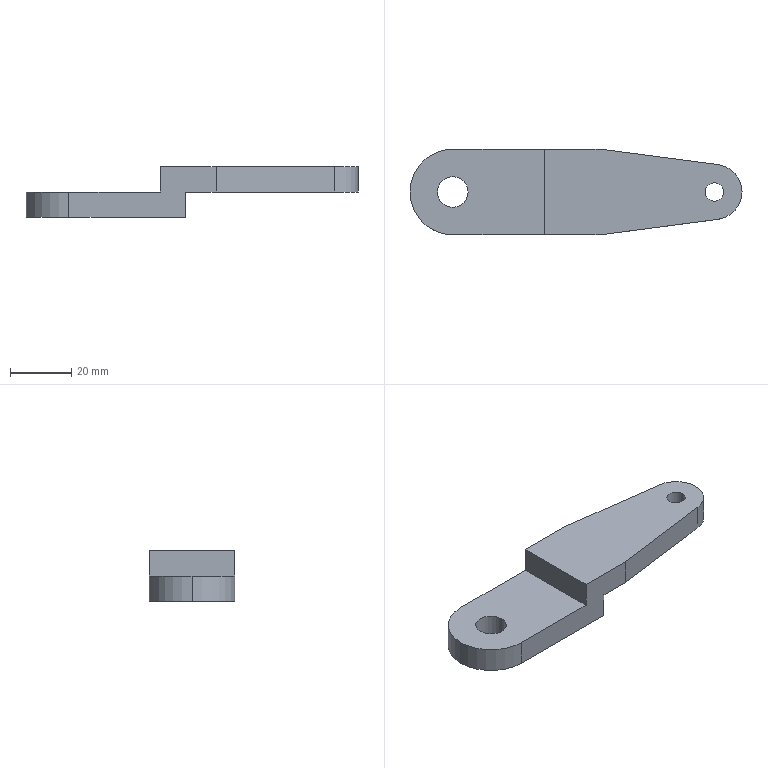Part | SolidWorks | features Extrusion 1, ICE 1 | 1 solid | 17 faces | box 108.5 x 28 x 16.6 mm | volume 22997 mm3 | plane 10 | cylinder 7 | commonest cylinder face diameters 6 x2 10 x2 28 x2 18 x1
STEP:
#1=CARTESIAN_POINT('',(52.6,0.,16.6));
#2=VERTEX_POINT('',#1);
#3=CARTESIAN_POINT('',(58.6,0.,16.6));
#4=VERTEX_POINT('',#3);
#5=CARTESIAN_POINT('',(55.6,0.,16.6));
#6=DIRECTION('',(0.,0.,1.));
#7=DIRECTION('',(1.,0.,0.));
#8=AXIS2_PLACEMENT_3D('',#5,#6,#7);
#9=CIRCLE('',#8,3.);
#10=EDGE_CURVE('',#2,#4,#9,.T.);
#11=ORIENTED_EDGE('',*,*,#10,.T.);
#12=CARTESIAN_POINT('',(58.6,0.,8.3));
#13=VERTEX_POINT('',#12);
#14=CARTESIAN_POINT('',(58.6,0.,16.6));
#15=DIRECTION('',(0.,0.,-1.));
#16=VECTOR('',#15,1000.);
#17=LINE('',#14,#16);
#18=EDGE_CURVE('',#4,#13,#17,.T.);
#19=ORIENTED_EDGE('',*,*,#18,.T.);
#20=CARTESIAN_POINT('',(52.6,0.,8.3));
#21=VERTEX_POINT('',#20);
#22=CARTESIAN_POINT('',(55.6,0.,8.3));
#23=DIRECTION('',(0.,0.,1.));
#24=DIRECTION('',(1.,0.,0.));
#25=AXIS2_PLACEMENT_3D('',#22,#23,#24);
#26=CIRCLE('',#25,3.);
#27=EDGE_CURVE('',#21,#13,#26,.T.);
#28=ORIENTED_EDGE('',*,*,#27,.F.);
#29=CARTESIAN_POINT('',(52.6,0.,16.6));
#30=DIRECTION('',(0.,0.,-1.));
#31=VECTOR('',#30,1000.);
#32=LINE('',#29,#31);
#33=EDGE_CURVE('',#2,#21,#32,.T.);
#34=ORIENTED_EDGE('',*,*,#33,.F.);
#35=EDGE_LOOP('',(#11,#19,#28,#34));
#36=FACE_OUTER_BOUND('',#35,.T.);
#37=CARTESIAN_POINT('',(55.6,0.,16.6));
#38=DIRECTION('',(0.,0.,-1.));
#39=DIRECTION('',(-1.,0.,0.));
#40=AXIS2_PLACEMENT_3D('',#37,#38,#39);
#41=CYLINDRICAL_SURFACE('',#40,3.);
#42=ADVANCED_FACE('',(#36),#41,.F.);
#43=CARTESIAN_POINT('',(-34.9,0.,8.3));
#44=VERTEX_POINT('',#43);
#45=CARTESIAN_POINT('',(-24.9,0.,8.3));
#46=VERTEX_POINT('',#45);
#47=CARTESIAN_POINT('',(-29.9,0.,8.3));
#48=DIRECTION('',(0.,0.,1.));
#49=DIRECTION('',(1.,0.,0.));
#50=AXIS2_PLACEMENT_3D('',#47,#48,#49);
#51=CIRCLE('',#50,5.);
#52=EDGE_CURVE('',#44,#46,#51,.T.);
#53=ORIENTED_EDGE('',*,*,#52,.T.);
#54=CARTESIAN_POINT('',(-24.9,0.,0.));
#55=VERTEX_POINT('',#54);
#56=CARTESIAN_POINT('',(-24.9,0.,8.3));
#57=DIRECTION('',(0.,0.,-1.));
#58=VECTOR('',#57,1000.);
#59=LINE('',#56,#58);
#60=EDGE_CURVE('',#46,#55,#59,.T.);
#61=ORIENTED_EDGE('',*,*,#60,.T.);
#62=CARTESIAN_POINT('',(-34.9,0.,0.));
#63=VERTEX_POINT('',#62);
#64=CARTESIAN_POINT('',(-29.9,0.,0.));
#65=DIRECTION('',(0.,0.,1.));
#66=DIRECTION('',(1.,0.,0.));
#67=AXIS2_PLACEMENT_3D('',#64,#65,#66);
#68=CIRCLE('',#67,5.);
#69=EDGE_CURVE('',#63,#55,#68,.T.);
#70=ORIENTED_EDGE('',*,*,#69,.F.);
#71=CARTESIAN_POINT('',(-34.9,0.,8.3));
#72=DIRECTION('',(0.,0.,-1.));
#73=VECTOR('',#72,1000.);
#74=LINE('',#71,#73);
#75=EDGE_CURVE('',#44,#63,#74,.T.);
#76=ORIENTED_EDGE('',*,*,#75,.F.);
#77=EDGE_LOOP('',(#53,#61,#70,#76));
#78=FACE_OUTER_BOUND('',#77,.T.);
#79=CARTESIAN_POINT('',(-29.9,0.,8.3));
#80=DIRECTION('',(0.,0.,-1.));
#81=DIRECTION('',(-1.,0.,0.));
#82=AXIS2_PLACEMENT_3D('',#79,#80,#81);
#83=CYLINDRICAL_SURFACE('',#82,5.);
#84=ADVANCED_FACE('',(#78),#83,.F.);
#85=CARTESIAN_POINT('',(-43.9,0.,8.3));
#86=VERTEX_POINT('',#85);
#87=CARTESIAN_POINT('',(-29.9,-14.,8.3));
#88=VERTEX_POINT('',#87);
#89=CARTESIAN_POINT('',(-29.9,0.,8.3));
#90=DIRECTION('',(0.,0.,1.));
#91=DIRECTION('',(1.,0.,0.));
#92=AXIS2_PLACEMENT_3D('',#89,#90,#91);
#93=CIRCLE('',#92,14.);
#94=EDGE_CURVE('',#86,#88,#93,.T.);
#95=ORIENTED_EDGE('',*,*,#94,.F.);
#96=CARTESIAN_POINT('',(-43.9,0.,0.));
#97=VERTEX_POINT('',#96);
#98=CARTESIAN_POINT('',(-43.9,0.,8.3));
#99=DIRECTION('',(0.,0.,-1.));
#100=VECTOR('',#99,1000.);
#101=LINE('',#98,#100);
#102=EDGE_CURVE('',#86,#97,#101,.T.);
#103=ORIENTED_EDGE('',*,*,#102,.T.);
#104=CARTESIAN_POINT('',(-29.9,-14.,0.));
#105=VERTEX_POINT('',#104);
#106=CARTESIAN_POINT('',(-29.9,0.,0.));
#107=DIRECTION('',(0.,0.,1.));
#108=DIRECTION('',(1.,0.,0.));
#109=AXIS2_PLACEMENT_3D('',#106,#107,#108);
#110=CIRCLE('',#109,14.);
#111=EDGE_CURVE('',#97,#105,#110,.T.);
#112=ORIENTED_EDGE('',*,*,#111,.T.);
#113=CARTESIAN_POINT('',(-29.9,-14.,8.3));
#114=DIRECTION('',(0.,0.,-1.));
#115=VECTOR('',#114,1000.);
#116=LINE('',#113,#115);
#117=EDGE_CURVE('',#88,#105,#116,.T.);
#118=ORIENTED_EDGE('',*,*,#117,.F.);
#119=EDGE_LOOP('',(#95,#103,#112,#118));
#120=FACE_OUTER_BOUND('',#119,.T.);
#121=CARTESIAN_POINT('',(-29.9,0.,8.3));
#122=DIRECTION('',(0.,0.,-1.));
#123=DIRECTION('',(-1.,0.,0.));
#124=AXIS2_PLACEMENT_3D('',#121,#122,#123);
#125=CYLINDRICAL_SURFACE('',#124,14.);
#126=ADVANCED_FACE('',(#120),#125,.T.);
#127=CARTESIAN_POINT('',(-29.9,14.,0.));
#128=VERTEX_POINT('',#127);
#129=CARTESIAN_POINT('',(8.3,14.,0.));
#130=VERTEX_POINT('',#129);
#131=CARTESIAN_POINT('',(0.,14.,0.));
#132=DIRECTION('',(1.,0.,0.));
#133=VECTOR('',#132,1000.);
#134=LINE('',#131,#133);
#135=EDGE_CURVE('',#128,#130,#134,.T.);
#136=ORIENTED_EDGE('',*,*,#135,.F.);
#137=CARTESIAN_POINT('',(-29.9,14.,8.3));
#138=VERTEX_POINT('',#137);
#139=CARTESIAN_POINT('',(-29.9,14.,8.3));
#140=DIRECTION('',(0.,0.,-1.));
#141=VECTOR('',#140,1000.);
#142=LINE('',#139,#141);
#143=EDGE_CURVE('',#138,#128,#142,.T.);
#144=ORIENTED_EDGE('',*,*,#143,.F.);
#145=CARTESIAN_POINT('',(0.,14.,8.3));
#146=VERTEX_POINT('',#145);
#147=CARTESIAN_POINT('',(0.,14.,8.3));
#148=DIRECTION('',(1.,0.,0.));
#149=VECTOR('',#148,1000.);
#150=LINE('',#147,#149);
#151=EDGE_CURVE('',#138,#146,#150,.T.);
#152=ORIENTED_EDGE('',*,*,#151,.T.);
#153=CARTESIAN_POINT('',(0.,14.,16.6));
#154=VERTEX_POINT('',#153);
#155=CARTESIAN_POINT('',(0.,14.,16.6));
#156=DIRECTION('',(0.,0.,-1.));
#157=VECTOR('',#156,1000.);
#158=LINE('',#155,#157);
#159=EDGE_CURVE('',#154,#146,#158,.T.);
#160=ORIENTED_EDGE('',*,*,#159,.F.);
#161=CARTESIAN_POINT('',(18.211,14.,16.6));
#162=VERTEX_POINT('',#161);
#163=CARTESIAN_POINT('',(0.,14.,16.6));
#164=DIRECTION('',(-1.,0.,0.));
#165=VECTOR('',#164,1000.);
#166=LINE('',#163,#165);
#167=EDGE_CURVE('',#162,#154,#166,.T.);
#168=ORIENTED_EDGE('',*,*,#167,.F.);
#169=CARTESIAN_POINT('',(18.211,14.,8.3));
#170=VERTEX_POINT('',#169);
#171=CARTESIAN_POINT('',(18.211,14.,16.6));
#172=DIRECTION('',(0.,0.,-1.));
#173=VECTOR('',#172,1000.);
#174=LINE('',#171,#173);
#175=EDGE_CURVE('',#162,#170,#174,.T.);
#176=ORIENTED_EDGE('',*,*,#175,.T.);
#177=CARTESIAN_POINT('',(8.3,14.,8.3));
#178=VERTEX_POINT('',#177);
#179=CARTESIAN_POINT('',(0.,14.,8.3));
#180=DIRECTION('',(-1.,0.,0.));
#181=VECTOR('',#180,1000.);
#182=LINE('',#179,#181);
#183=EDGE_CURVE('',#170,#178,#182,.T.);
#184=ORIENTED_EDGE('',*,*,#183,.T.);
#185=CARTESIAN_POINT('',(8.3,14.,8.3));
#186=DIRECTION('',(0.,0.,-1.));
#187=VECTOR('',#186,1000.);
#188=LINE('',#185,#187);
#189=EDGE_CURVE('',#178,#130,#188,.T.);
#190=ORIENTED_EDGE('',*,*,#189,.T.);
#191=EDGE_LOOP('',(#136,#144,#152,#160,#168,#176,#184,#190));
#192=FACE_OUTER_BOUND('',#191,.T.);
#193=CARTESIAN_POINT('',(0.,14.,8.3));
#194=DIRECTION('',(0.,1.,0.));
#195=DIRECTION('',(0.,0.,1.));
#196=AXIS2_PLACEMENT_3D('',#193,#194,#195);
#197=PLANE('',#196);
#198=ADVANCED_FACE('',(#192),#197,.T.);
#199=ORIENTED_EDGE('',*,*,#102,.F.);
#200=CARTESIAN_POINT('',(-29.9,0.,8.3));
#201=DIRECTION('',(0.,0.,1.));
#202=DIRECTION('',(1.,0.,0.));
#203=AXIS2_PLACEMENT_3D('',#200,#201,#202);
#204=CIRCLE('',#203,14.);
#205=EDGE_CURVE('',#138,#86,#204,.T.);
#206=ORIENTED_EDGE('',*,*,#205,.F.);
#207=ORIENTED_EDGE('',*,*,#143,.T.);
#208=CARTESIAN_POINT('',(-29.9,0.,0.));
#209=DIRECTION('',(0.,0.,1.));
#210=DIRECTION('',(1.,0.,0.));
#211=AXIS2_PLACEMENT_3D('',#208,#209,#210);
#212=CIRCLE('',#211,14.);
#213=EDGE_CURVE('',#128,#97,#212,.T.);
#214=ORIENTED_EDGE('',*,*,#213,.T.);
#215=EDGE_LOOP('',(#199,#206,#207,#214));
#216=FACE_OUTER_BOUND('',#215,.T.);
#217=CARTESIAN_POINT('',(-29.9,0.,8.3));
#218=DIRECTION('',(0.,0.,-1.));
#219=DIRECTION('',(-1.,0.,0.));
#220=AXIS2_PLACEMENT_3D('',#217,#218,#219);
#221=CYLINDRICAL_SURFACE('',#220,14.);
#222=ADVANCED_FACE('',(#216),#221,.T.);
#223=CARTESIAN_POINT('',(8.3,-14.,0.));
#224=VERTEX_POINT('',#223);
#225=CARTESIAN_POINT('',(0.,-14.,0.));
#226=DIRECTION('',(1.,0.,0.));
#227=VECTOR('',#226,1000.);
#228=LINE('',#225,#227);
#229=EDGE_CURVE('',#105,#224,#228,.T.);
#230=ORIENTED_EDGE('',*,*,#229,.T.);
#231=CARTESIAN_POINT('',(8.3,-14.,8.3));
#232=VERTEX_POINT('',#231);
#233=CARTESIAN_POINT('',(8.3,-14.,8.3));
#234=DIRECTION('',(0.,0.,-1.));
#235=VECTOR('',#234,1000.);
#236=LINE('',#233,#235);
#237=EDGE_CURVE('',#232,#224,#236,.T.);
#238=ORIENTED_EDGE('',*,*,#237,.F.);
#239=CARTESIAN_POINT('',(18.211,-14.,8.3));
#240=VERTEX_POINT('',#239);
#241=CARTESIAN_POINT('',(0.,-14.,8.3));
#242=DIRECTION('',(1.,0.,0.));
#243=VECTOR('',#242,1000.);
#244=LINE('',#241,#243);
#245=EDGE_CURVE('',#232,#240,#244,.T.);
#246=ORIENTED_EDGE('',*,*,#245,.T.);
#247=CARTESIAN_POINT('',(18.211,-14.,16.6));
#248=VERTEX_POINT('',#247);
#249=CARTESIAN_POINT('',(18.211,-14.,16.6));
#250=DIRECTION('',(0.,0.,-1.));
#251=VECTOR('',#250,1000.);
#252=LINE('',#249,#251);
#253=EDGE_CURVE('',#248,#240,#252,.T.);
#254=ORIENTED_EDGE('',*,*,#253,.F.);
#255=CARTESIAN_POINT('',(0.,-14.,16.6));
#256=VERTEX_POINT('',#255);
#257=CARTESIAN_POINT('',(0.,-14.,16.6));
#258=DIRECTION('',(1.,0.,0.));
#259=VECTOR('',#258,1000.);
#260=LINE('',#257,#259);
#261=EDGE_CURVE('',#256,#248,#260,.T.);
#262=ORIENTED_EDGE('',*,*,#261,.F.);
#263=CARTESIAN_POINT('',(0.,-14.,8.3));
#264=VERTEX_POINT('',#263);
#265=CARTESIAN_POINT('',(0.,-14.,16.6));
#266=DIRECTION('',(0.,0.,-1.));
#267=VECTOR('',#266,1000.);
#268=LINE('',#265,#267);
#269=EDGE_CURVE('',#256,#264,#268,.T.);
#270=ORIENTED_EDGE('',*,*,#269,.T.);
#271=CARTESIAN_POINT('',(0.,-14.,8.3));
#272=DIRECTION('',(1.,0.,0.));
#273=VECTOR('',#272,1000.);
#274=LINE('',#271,#273);
#275=EDGE_CURVE('',#88,#264,#274,.T.);
#276=ORIENTED_EDGE('',*,*,#275,.F.);
#277=ORIENTED_EDGE('',*,*,#117,.T.);
#278=EDGE_LOOP('',(#230,#238,#246,#254,#262,#270,#276,#277));
#279=FACE_OUTER_BOUND('',#278,.T.);
#280=CARTESIAN_POINT('',(0.,-14.,8.3));
#281=DIRECTION('',(0.,1.,0.));
#282=DIRECTION('',(0.,0.,1.));
#283=AXIS2_PLACEMENT_3D('',#280,#281,#282);
#284=PLANE('',#283);
#285=ADVANCED_FACE('',(#279),#284,.F.);
#286=ORIENTED_EDGE('',*,*,#60,.F.);
#287=CARTESIAN_POINT('',(-29.9,0.,8.3));
#288=DIRECTION('',(0.,0.,1.));
#289=DIRECTION('',(1.,0.,0.));
#290=AXIS2_PLACEMENT_3D('',#287,#288,#289);
#291=CIRCLE('',#290,5.);
#292=EDGE_CURVE('',#46,#44,#291,.T.);
#293=ORIENTED_EDGE('',*,*,#292,.T.);
#294=ORIENTED_EDGE('',*,*,#75,.T.);
#295=CARTESIAN_POINT('',(-29.9,0.,0.));
#296=DIRECTION('',(0.,0.,1.));
#297=DIRECTION('',(1.,0.,0.));
#298=AXIS2_PLACEMENT_3D('',#295,#296,#297);
#299=CIRCLE('',#298,5.);
#300=EDGE_CURVE('',#55,#63,#299,.T.);
#301=ORIENTED_EDGE('',*,*,#300,.F.);
#302=EDGE_LOOP('',(#286,#293,#294,#301));
#303=FACE_OUTER_BOUND('',#302,.T.);
#304=CARTESIAN_POINT('',(-29.9,0.,8.3));
#305=DIRECTION('',(0.,0.,-1.));
#306=DIRECTION('',(-1.,0.,0.));
#307=AXIS2_PLACEMENT_3D('',#304,#305,#306);
#308=CYLINDRICAL_SURFACE('',#307,5.);
#309=ADVANCED_FACE('',(#303),#308,.F.);
#310=CARTESIAN_POINT('',(8.3,0.,0.));
#311=DIRECTION('',(0.,-1.,0.));
#312=VECTOR('',#311,1000.);
#313=LINE('',#310,#312);
#314=EDGE_CURVE('',#130,#224,#313,.T.);
#315=ORIENTED_EDGE('',*,*,#314,.F.);
#316=ORIENTED_EDGE('',*,*,#189,.F.);
#317=CARTESIAN_POINT('',(8.3,0.,8.3));
#318=DIRECTION('',(0.,-1.,0.));
#319=VECTOR('',#318,1000.);
#320=LINE('',#317,#319);
#321=EDGE_CURVE('',#178,#232,#320,.T.);
#322=ORIENTED_EDGE('',*,*,#321,.T.);
#323=ORIENTED_EDGE('',*,*,#237,.T.);
#324=EDGE_LOOP('',(#315,#316,#322,#323));
#325=FACE_OUTER_BOUND('',#324,.T.);
#326=CARTESIAN_POINT('',(8.3,0.,8.3));
#327=DIRECTION('',(1.,0.,0.));
#328=DIRECTION('',(0.,0.,-1.));
#329=AXIS2_PLACEMENT_3D('',#326,#327,#328);
#330=PLANE('',#329);
#331=ADVANCED_FACE('',(#325),#330,.T.);
#332=CARTESIAN_POINT('',(0.,14.,8.3));
#333=DIRECTION('',(0.,-1.,0.));
#334=VECTOR('',#333,1000.);
#335=LINE('',#332,#334);
#336=EDGE_CURVE('',#146,#264,#335,.T.);
#337=ORIENTED_EDGE('',*,*,#336,.F.);
#338=ORIENTED_EDGE('',*,*,#151,.F.);
#339=ORIENTED_EDGE('',*,*,#205,.T.);
#340=ORIENTED_EDGE('',*,*,#94,.T.);
#341=ORIENTED_EDGE('',*,*,#275,.T.);
#342=EDGE_LOOP('',(#337,#338,#339,#340,#341));
#343=FACE_OUTER_BOUND('',#342,.T.);
#344=ORIENTED_EDGE('',*,*,#52,.F.);
#345=ORIENTED_EDGE('',*,*,#292,.F.);
#346=EDGE_LOOP('',(#344,#345));
#347=FACE_BOUND('',#346,.T.);
#348=CARTESIAN_POINT('',(0.,0.,8.3));
#349=DIRECTION('',(0.,0.,1.));
#350=DIRECTION('',(1.,0.,0.));
#351=AXIS2_PLACEMENT_3D('',#348,#349,#350);
#352=PLANE('',#351);
#353=ADVANCED_FACE('',(#343,#347),#352,.T.);
#354=ORIENTED_EDGE('',*,*,#69,.T.);
#355=ORIENTED_EDGE('',*,*,#300,.T.);
#356=EDGE_LOOP('',(#354,#355));
#357=FACE_BOUND('',#356,.T.);
#358=ORIENTED_EDGE('',*,*,#135,.T.);
#359=ORIENTED_EDGE('',*,*,#314,.T.);
#360=ORIENTED_EDGE('',*,*,#229,.F.);
#361=ORIENTED_EDGE('',*,*,#111,.F.);
#362=ORIENTED_EDGE('',*,*,#213,.F.);
#363=EDGE_LOOP('',(#358,#359,#360,#361,#362));
#364=FACE_OUTER_BOUND('',#363,.T.);
#365=CARTESIAN_POINT('',(0.,0.,0.));
#366=DIRECTION('',(0.,0.,1.));
#367=DIRECTION('',(1.,0.,0.));
#368=AXIS2_PLACEMENT_3D('',#365,#366,#367);
#369=PLANE('',#368);
#370=ADVANCED_FACE('',(#357,#364),#369,.F.);
#371=ORIENTED_EDGE('',*,*,#167,.T.);
#372=CARTESIAN_POINT('',(0.,14.,16.6));
#373=DIRECTION('',(0.,-1.,0.));
#374=VECTOR('',#373,1000.);
#375=LINE('',#372,#374);
#376=EDGE_CURVE('',#154,#256,#375,.T.);
#377=ORIENTED_EDGE('',*,*,#376,.T.);
#378=ORIENTED_EDGE('',*,*,#261,.T.);
#379=CARTESIAN_POINT('',(56.775,-8.923,16.6));
#380=VERTEX_POINT('',#379);
#381=CARTESIAN_POINT('',(18.211,-14.,16.6));
#382=DIRECTION('',(0.9914,0.1305,0.));
#383=VECTOR('',#382,1000.);
#384=LINE('',#381,#383);
#385=EDGE_CURVE('',#248,#380,#384,.T.);
#386=ORIENTED_EDGE('',*,*,#385,.T.);
#387=CARTESIAN_POINT('',(56.775,8.923,16.6));
#388=VERTEX_POINT('',#387);
#389=CARTESIAN_POINT('',(55.6,0.,16.6));
#390=DIRECTION('',(0.,0.,1.));
#391=DIRECTION('',(1.,0.,0.));
#392=AXIS2_PLACEMENT_3D('',#389,#390,#391);
#393=CIRCLE('',#392,9.);
#394=EDGE_CURVE('',#380,#388,#393,.T.);
#395=ORIENTED_EDGE('',*,*,#394,.T.);
#396=CARTESIAN_POINT('',(18.211,14.,16.6));
#397=DIRECTION('',(-0.9914,0.1305,0.));
#398=VECTOR('',#397,1000.);
#399=LINE('',#396,#398);
#400=EDGE_CURVE('',#388,#162,#399,.T.);
#401=ORIENTED_EDGE('',*,*,#400,.T.);
#402=EDGE_LOOP('',(#371,#377,#378,#386,#395,#401));
#403=FACE_OUTER_BOUND('',#402,.T.);
#404=ORIENTED_EDGE('',*,*,#10,.F.);
#405=CARTESIAN_POINT('',(55.6,0.,16.6));
#406=DIRECTION('',(0.,0.,1.));
#407=DIRECTION('',(1.,0.,0.));
#408=AXIS2_PLACEMENT_3D('',#405,#406,#407);
#409=CIRCLE('',#408,3.);
#410=EDGE_CURVE('',#4,#2,#409,.T.);
#411=ORIENTED_EDGE('',*,*,#410,.F.);
#412=EDGE_LOOP('',(#404,#411));
#413=FACE_BOUND('',#412,.T.);
#414=CARTESIAN_POINT('',(55.6,0.,16.6));
#415=DIRECTION('',(0.,0.,1.));
#416=DIRECTION('',(1.,0.,0.));
#417=AXIS2_PLACEMENT_3D('',#414,#415,#416);
#418=PLANE('',#417);
#419=ADVANCED_FACE('',(#403,#413),#418,.T.);
#420=ORIENTED_EDGE('',*,*,#321,.F.);
#421=ORIENTED_EDGE('',*,*,#183,.F.);
#422=CARTESIAN_POINT('',(56.775,8.923,8.3));
#423=VERTEX_POINT('',#422);
#424=CARTESIAN_POINT('',(18.211,14.,8.3));
#425=DIRECTION('',(-0.9914,0.1305,0.));
#426=VECTOR('',#425,1000.);
#427=LINE('',#424,#426);
#428=EDGE_CURVE('',#423,#170,#427,.T.);
#429=ORIENTED_EDGE('',*,*,#428,.F.);
#430=CARTESIAN_POINT('',(56.775,-8.923,8.3));
#431=VERTEX_POINT('',#430);
#432=CARTESIAN_POINT('',(55.6,0.,8.3));
#433=DIRECTION('',(0.,0.,1.));
#434=DIRECTION('',(1.,0.,0.));
#435=AXIS2_PLACEMENT_3D('',#432,#433,#434);
#436=CIRCLE('',#435,9.);
#437=EDGE_CURVE('',#431,#423,#436,.T.);
#438=ORIENTED_EDGE('',*,*,#437,.F.);
#439=CARTESIAN_POINT('',(18.211,-14.,8.3));
#440=DIRECTION('',(0.9914,0.1305,0.));
#441=VECTOR('',#440,1000.);
#442=LINE('',#439,#441);
#443=EDGE_CURVE('',#240,#431,#442,.T.);
#444=ORIENTED_EDGE('',*,*,#443,.F.);
#445=ORIENTED_EDGE('',*,*,#245,.F.);
#446=EDGE_LOOP('',(#420,#421,#429,#438,#444,#445));
#447=FACE_OUTER_BOUND('',#446,.T.);
#448=ORIENTED_EDGE('',*,*,#27,.T.);
#449=CARTESIAN_POINT('',(55.6,0.,8.3));
#450=DIRECTION('',(0.,0.,1.));
#451=DIRECTION('',(1.,0.,0.));
#452=AXIS2_PLACEMENT_3D('',#449,#450,#451);
#453=CIRCLE('',#452,3.);
#454=EDGE_CURVE('',#13,#21,#453,.T.);
#455=ORIENTED_EDGE('',*,*,#454,.T.);
#456=EDGE_LOOP('',(#448,#455));
#457=FACE_BOUND('',#456,.T.);
#458=CARTESIAN_POINT('',(55.6,0.,8.3));
#459=DIRECTION('',(0.,0.,1.));
#460=DIRECTION('',(1.,0.,0.));
#461=AXIS2_PLACEMENT_3D('',#458,#459,#460);
#462=PLANE('',#461);
#463=ADVANCED_FACE('',(#447,#457),#462,.F.);
#464=ORIENTED_EDGE('',*,*,#336,.T.);
#465=ORIENTED_EDGE('',*,*,#269,.F.);
#466=ORIENTED_EDGE('',*,*,#376,.F.);
#467=ORIENTED_EDGE('',*,*,#159,.T.);
#468=EDGE_LOOP('',(#464,#465,#466,#467));
#469=FACE_OUTER_BOUND('',#468,.T.);
#470=CARTESIAN_POINT('',(0.,14.,16.6));
#471=DIRECTION('',(1.,0.,0.));
#472=DIRECTION('',(0.,0.,-1.));
#473=AXIS2_PLACEMENT_3D('',#470,#471,#472);
#474=PLANE('',#473);
#475=ADVANCED_FACE('',(#469),#474,.F.);
#476=ORIENTED_EDGE('',*,*,#443,.T.);
#477=CARTESIAN_POINT('',(56.775,-8.923,16.6));
#478=DIRECTION('',(0.,0.,-1.));
#479=VECTOR('',#478,1000.);
#480=LINE('',#477,#479);
#481=EDGE_CURVE('',#380,#431,#480,.T.);
#482=ORIENTED_EDGE('',*,*,#481,.F.);
#483=ORIENTED_EDGE('',*,*,#385,.F.);
#484=ORIENTED_EDGE('',*,*,#253,.T.);
#485=EDGE_LOOP('',(#476,#482,#483,#484));
#486=FACE_OUTER_BOUND('',#485,.T.);
#487=CARTESIAN_POINT('',(18.211,-14.,16.6));
#488=DIRECTION('',(-0.1305,0.9914,0.));
#489=DIRECTION('',(-0.9914,-0.1305,0.));
#490=AXIS2_PLACEMENT_3D('',#487,#488,#489);
#491=PLANE('',#490);
#492=ADVANCED_FACE('',(#486),#491,.F.);
#493=ORIENTED_EDGE('',*,*,#437,.T.);
#494=CARTESIAN_POINT('',(56.775,8.923,16.6));
#495=DIRECTION('',(0.,0.,-1.));
#496=VECTOR('',#495,1000.);
#497=LINE('',#494,#496);
#498=EDGE_CURVE('',#388,#423,#497,.T.);
#499=ORIENTED_EDGE('',*,*,#498,.F.);
#500=ORIENTED_EDGE('',*,*,#394,.F.);
#501=ORIENTED_EDGE('',*,*,#481,.T.);
#502=EDGE_LOOP('',(#493,#499,#500,#501));
#503=FACE_OUTER_BOUND('',#502,.T.);
#504=CARTESIAN_POINT('',(55.6,0.,16.6));
#505=DIRECTION('',(0.,0.,-1.));
#506=DIRECTION('',(-1.,0.,0.));
#507=AXIS2_PLACEMENT_3D('',#504,#505,#506);
#508=CYLINDRICAL_SURFACE('',#507,9.);
#509=ADVANCED_FACE('',(#503),#508,.T.);
#510=ORIENTED_EDGE('',*,*,#428,.T.);
#511=ORIENTED_EDGE('',*,*,#175,.F.);
#512=ORIENTED_EDGE('',*,*,#400,.F.);
#513=ORIENTED_EDGE('',*,*,#498,.T.);
#514=EDGE_LOOP('',(#510,#511,#512,#513));
#515=FACE_OUTER_BOUND('',#514,.T.);
#516=CARTESIAN_POINT('',(18.211,14.,16.6));
#517=DIRECTION('',(-0.1305,-0.9914,0.));
#518=DIRECTION('',(0.9914,-0.1305,0.));
#519=AXIS2_PLACEMENT_3D('',#516,#517,#518);
#520=PLANE('',#519);
#521=ADVANCED_FACE('',(#515),#520,.F.);
#522=ORIENTED_EDGE('',*,*,#18,.F.);
#523=ORIENTED_EDGE('',*,*,#410,.T.);
#524=ORIENTED_EDGE('',*,*,#33,.T.);
#525=ORIENTED_EDGE('',*,*,#454,.F.);
#526=EDGE_LOOP('',(#522,#523,#524,#525));
#527=FACE_OUTER_BOUND('',#526,.T.);
#528=CARTESIAN_POINT('',(55.6,0.,16.6));
#529=DIRECTION('',(0.,0.,-1.));
#530=DIRECTION('',(-1.,0.,0.));
#531=AXIS2_PLACEMENT_3D('',#528,#529,#530);
#532=CYLINDRICAL_SURFACE('',#531,3.);
#533=ADVANCED_FACE('',(#527),#532,.F.);
#534=CLOSED_SHELL('',(#42,#84,#126,#198,#222,#285,#309,#331,#353,#370,#419,#463,#475,#492,#509,#521,#533));
#535=MANIFOLD_SOLID_BREP('',#534);
#536=CARTESIAN_POINT('',(0.,0.,0.));
#537=DIRECTION('',(0.,0.,1.));
#538=DIRECTION('',(1.,0.,0.));
#539=AXIS2_PLACEMENT_3D('',#536,#537,#538);
#540=(LENGTH_UNIT()NAMED_UNIT(*)SI_UNIT(.MILLI.,.METRE.));
#541=UNCERTAINTY_MEASURE_WITH_UNIT(LENGTH_MEASURE(0.00001),#540,'','');
#542=(NAMED_UNIT(*)PLANE_ANGLE_UNIT()SI_UNIT($,.RADIAN.));
#543=(NAMED_UNIT(*)SI_UNIT($,.STERADIAN.)SOLID_ANGLE_UNIT());
#544=(GEOMETRIC_REPRESENTATION_CONTEXT(3)GLOBAL_UNCERTAINTY_ASSIGNED_CONTEXT((#541))GLOBAL_UNIT_ASSIGNED_CONTEXT((#540,#542,#543))REPRESENTATION_CONTEXT('',''));
#545=ADVANCED_BREP_SHAPE_REPRESENTATION('',(#535,#539),#544);